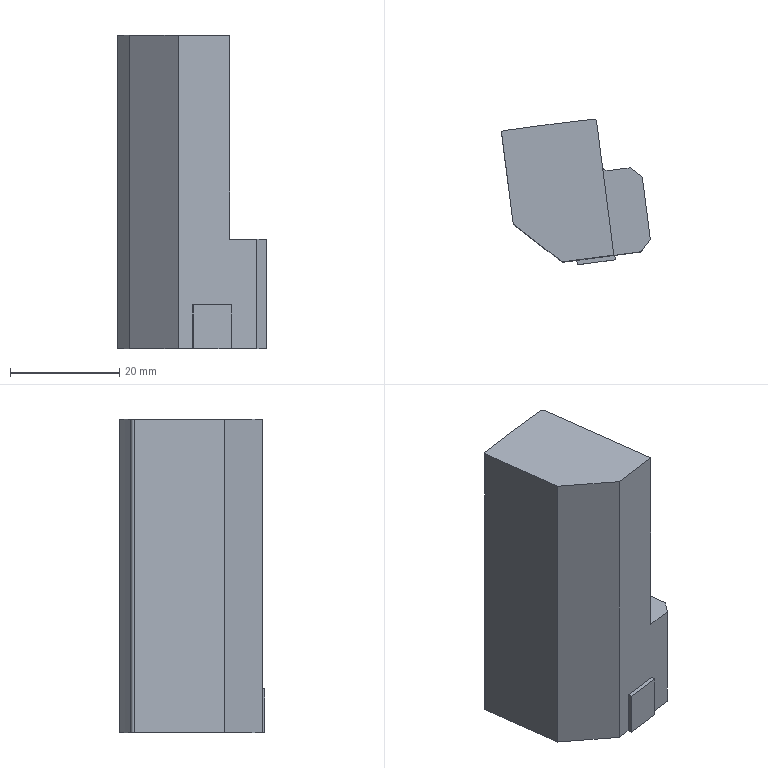Part | STEP file | gslz 2016.10.28-13_id294_x_t | 1 solid | 19 faces | box 27.194 x 26.527 x 57.25 mm | volume 25529 mm3 | plane 15 | cylinder 3 | other 1 | commonest cylinder face diameters 1 x2 2 x1